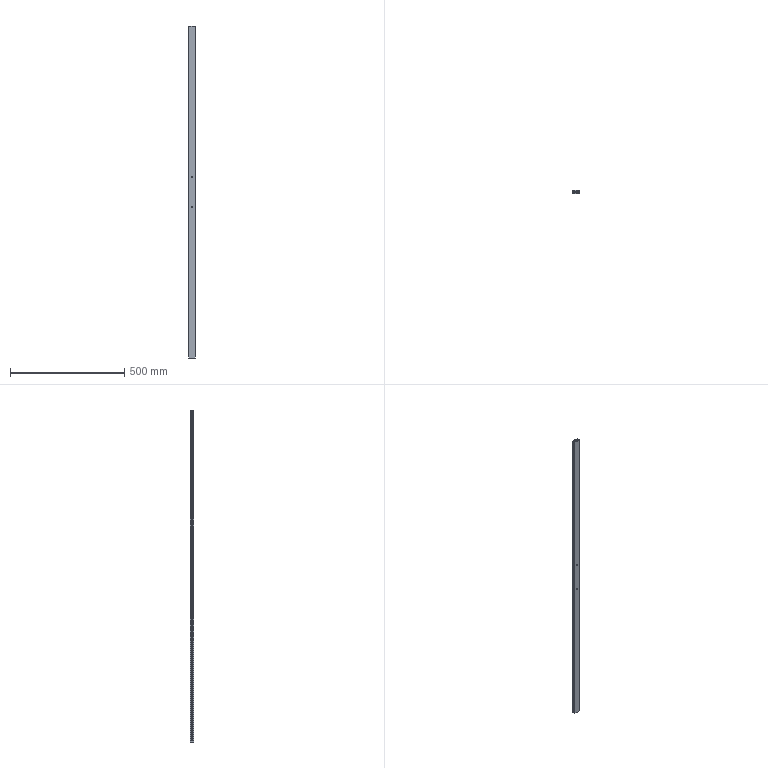Part | SolidWorks | features HoleWzd 3, BaseBody 1, MoveFace 1 | 1 solid | 176 faces | box 30 x 15 x 1456 mm | volume 350164 mm3 | cylinder 88 | plane 72 | cone 16 | commonest cylinder face diameters 5 x26 3.3 x24 4.5 x16 1 x12 2 x4 6.6 x4